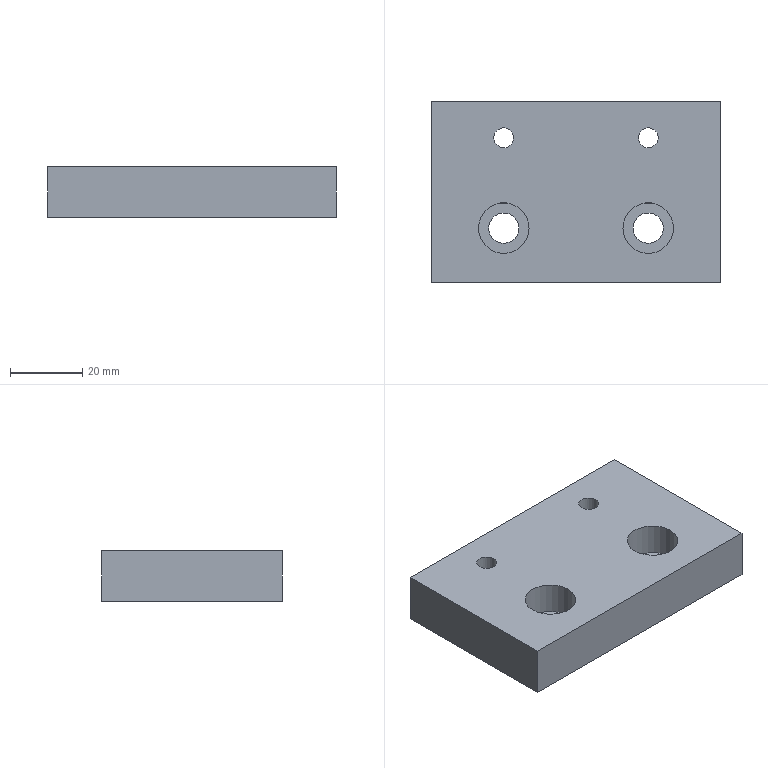Part | STEP file | 1 solid | 18 faces | box 80 x 50 x 14 mm | volume 51452 mm3 | plane 10 | cylinder 8 | commonest cylinder face diameters 5.5 x2 8.4 x2 9 x2 14 x2
STEP:
#1=CARTESIAN_POINT('',(0.,0.,0.));
#2=DIRECTION('',(0.,0.,1.));
#3=DIRECTION('',(1.,0.,0.));
#4=AXIS2_PLACEMENT_3D('',#1,#2,#3);
#5=CARTESIAN_POINT('',(57.147,-30.689,0.));
#6=VERTEX_POINT('',#5);
#7=CARTESIAN_POINT('',(52.947,-30.689,0.));
#8=DIRECTION('',(0.,0.,-1.));
#9=DIRECTION('',(1.,0.,0.));
#10=AXIS2_PLACEMENT_3D('',#7,#8,#9);
#11=CIRCLE('',#10,4.2);
#12=CARTESIAN_POINT('',(0.,0.,0.));
#13=DIRECTION('',(0.,0.,1.));
#14=DIRECTION('',(1.,0.,0.));
#15=AXIS2_PLACEMENT_3D('',#12,#13,#14);
#16=PLANE('',#15);
#17=CARTESIAN_POINT('',(57.147,-30.689));
#18=CARTESIAN_POINT('',(57.147,-37.964));
#19=CARTESIAN_POINT('',(50.847,-34.326));
#20=CARTESIAN_POINT('',(44.547,-30.689));
#21=CARTESIAN_POINT('',(50.847,-27.052));
#22=CARTESIAN_POINT('',(57.147,-23.414));
#23=CARTESIAN_POINT('',(57.147,-30.689));
#24=(BOUNDED_CURVE()B_SPLINE_CURVE(2,(#17,#18,#19,#20,#21,#22,#23),.UNSPECIFIED.,.T.,.F.)B_SPLINE_CURVE_WITH_KNOTS((1,2,2,2,2,1),(-2.094,0.,2.094,4.189,6.283,8.378),.UNSPECIFIED.)CURVE()GEOMETRIC_REPRESENTATION_ITEM()RATIONAL_B_SPLINE_CURVE((1.,0.5,1.,0.5,1.,0.5,1.))REPRESENTATION_ITEM(''));
#25=(GEOMETRIC_REPRESENTATION_CONTEXT(2)PARAMETRIC_REPRESENTATION_CONTEXT()REPRESENTATION_CONTEXT('',''));
#26=DEFINITIONAL_REPRESENTATION('',(#24),#25);
#27=PCURVE('',#16,#26);
#28=CARTESIAN_POINT('',(52.947,-30.689,14.));
#29=DIRECTION('',(0.,0.,1.));
#30=DIRECTION('',(1.,0.,0.));
#31=AXIS2_PLACEMENT_3D('',#28,#29,#30);
#32=CYLINDRICAL_SURFACE('',#31,4.2);
#33=CARTESIAN_POINT('',(6.283,-14.));
#34=DIRECTION('',(-1.,0.));
#35=VECTOR('',#34,1.);
#36=LINE('',#33,#35);
#37=(GEOMETRIC_REPRESENTATION_CONTEXT(2)PARAMETRIC_REPRESENTATION_CONTEXT()REPRESENTATION_CONTEXT('',''));
#38=DEFINITIONAL_REPRESENTATION('',(#36),#37);
#39=PCURVE('',#32,#38);
#40=SURFACE_CURVE('',#11,(#27,#39),.PCURVE_S1.);
#41=EDGE_CURVE('',#6,#6,#40,.T.);
#42=ORIENTED_EDGE('',*,*,#41,.F.);
#43=EDGE_LOOP('',(#42));
#44=FACE_BOUND('',#43,.T.);
#45=CARTESIAN_POINT('',(17.147,-30.689,0.));
#46=VERTEX_POINT('',#45);
#47=CARTESIAN_POINT('',(12.947,-30.689,0.));
#48=DIRECTION('',(0.,0.,-1.));
#49=DIRECTION('',(1.,0.,0.));
#50=AXIS2_PLACEMENT_3D('',#47,#48,#49);
#51=CIRCLE('',#50,4.2);
#52=CARTESIAN_POINT('',(17.147,-30.689));
#53=CARTESIAN_POINT('',(17.147,-37.964));
#54=CARTESIAN_POINT('',(10.847,-34.326));
#55=CARTESIAN_POINT('',(4.547,-30.689));
#56=CARTESIAN_POINT('',(10.847,-27.052));
#57=CARTESIAN_POINT('',(17.147,-23.414));
#58=CARTESIAN_POINT('',(17.147,-30.689));
#59=(BOUNDED_CURVE()B_SPLINE_CURVE(2,(#52,#53,#54,#55,#56,#57,#58),.UNSPECIFIED.,.T.,.F.)B_SPLINE_CURVE_WITH_KNOTS((1,2,2,2,2,1),(-2.094,0.,2.094,4.189,6.283,8.378),.UNSPECIFIED.)CURVE()GEOMETRIC_REPRESENTATION_ITEM()RATIONAL_B_SPLINE_CURVE((1.,0.5,1.,0.5,1.,0.5,1.))REPRESENTATION_ITEM(''));
#60=(GEOMETRIC_REPRESENTATION_CONTEXT(2)PARAMETRIC_REPRESENTATION_CONTEXT()REPRESENTATION_CONTEXT('',''));
#61=DEFINITIONAL_REPRESENTATION('',(#59),#60);
#62=PCURVE('',#16,#61);
#63=CARTESIAN_POINT('',(12.947,-30.689,14.));
#64=DIRECTION('',(0.,0.,1.));
#65=DIRECTION('',(1.,0.,0.));
#66=AXIS2_PLACEMENT_3D('',#63,#64,#65);
#67=CYLINDRICAL_SURFACE('',#66,4.2);
#68=CARTESIAN_POINT('',(6.283,-14.));
#69=DIRECTION('',(-1.,0.));
#70=VECTOR('',#69,1.);
#71=LINE('',#68,#70);
#72=(GEOMETRIC_REPRESENTATION_CONTEXT(2)PARAMETRIC_REPRESENTATION_CONTEXT()REPRESENTATION_CONTEXT('',''));
#73=DEFINITIONAL_REPRESENTATION('',(#71),#72);
#74=PCURVE('',#67,#73);
#75=SURFACE_CURVE('',#51,(#62,#74),.PCURVE_S1.);
#76=EDGE_CURVE('',#46,#46,#75,.T.);
#77=ORIENTED_EDGE('',*,*,#76,.F.);
#78=EDGE_LOOP('',(#77));
#79=FACE_BOUND('',#78,.T.);
#80=CARTESIAN_POINT('',(8.447,-5.689,0.));
#81=VERTEX_POINT('',#80);
#82=CARTESIAN_POINT('',(12.947,-5.689,0.));
#83=DIRECTION('',(0.,0.,-1.));
#84=DIRECTION('',(-1.,0.,0.));
#85=AXIS2_PLACEMENT_3D('',#82,#83,#84);
#86=CIRCLE('',#85,4.5);
#87=CARTESIAN_POINT('',(8.447,-5.689));
#88=CARTESIAN_POINT('',(8.447,2.105));
#89=CARTESIAN_POINT('',(15.197,-1.792));
#90=CARTESIAN_POINT('',(21.947,-5.689));
#91=CARTESIAN_POINT('',(15.197,-9.586));
#92=CARTESIAN_POINT('',(8.447,-13.483));
#93=CARTESIAN_POINT('',(8.447,-5.689));
#94=(BOUNDED_CURVE()B_SPLINE_CURVE(2,(#87,#88,#89,#90,#91,#92,#93),.UNSPECIFIED.,.T.,.F.)B_SPLINE_CURVE_WITH_KNOTS((1,2,2,2,2,1),(-2.094,0.,2.094,4.189,6.283,8.378),.UNSPECIFIED.)CURVE()GEOMETRIC_REPRESENTATION_ITEM()RATIONAL_B_SPLINE_CURVE((1.,0.5,1.,0.5,1.,0.5,1.))REPRESENTATION_ITEM(''));
#95=(GEOMETRIC_REPRESENTATION_CONTEXT(2)PARAMETRIC_REPRESENTATION_CONTEXT()REPRESENTATION_CONTEXT('',''));
#96=DEFINITIONAL_REPRESENTATION('',(#94),#95);
#97=PCURVE('',#16,#96);
#98=CARTESIAN_POINT('',(12.947,-5.689,0.));
#99=DIRECTION('',(0.,0.,-1.));
#100=DIRECTION('',(-1.,0.,0.));
#101=AXIS2_PLACEMENT_3D('',#98,#99,#100);
#102=CYLINDRICAL_SURFACE('',#101,4.5);
#103=CARTESIAN_POINT('',(0.,0.));
#104=DIRECTION('',(1.,0.));
#105=VECTOR('',#104,1.);
#106=LINE('',#103,#105);
#107=(GEOMETRIC_REPRESENTATION_CONTEXT(2)PARAMETRIC_REPRESENTATION_CONTEXT()REPRESENTATION_CONTEXT('',''));
#108=DEFINITIONAL_REPRESENTATION('',(#106),#107);
#109=PCURVE('',#102,#108);
#110=SURFACE_CURVE('',#86,(#97,#109),.PCURVE_S1.);
#111=EDGE_CURVE('',#81,#81,#110,.T.);
#112=ORIENTED_EDGE('',*,*,#111,.F.);
#113=EDGE_LOOP('',(#112));
#114=FACE_BOUND('',#113,.T.);
#115=CARTESIAN_POINT('',(48.447,-5.689,0.));
#116=VERTEX_POINT('',#115);
#117=CARTESIAN_POINT('',(52.947,-5.689,0.));
#118=DIRECTION('',(0.,0.,-1.));
#119=DIRECTION('',(-1.,0.,0.));
#120=AXIS2_PLACEMENT_3D('',#117,#118,#119);
#121=CIRCLE('',#120,4.5);
#122=CARTESIAN_POINT('',(48.447,-5.689));
#123=CARTESIAN_POINT('',(48.447,2.105));
#124=CARTESIAN_POINT('',(55.197,-1.792));
#125=CARTESIAN_POINT('',(61.947,-5.689));
#126=CARTESIAN_POINT('',(55.197,-9.586));
#127=CARTESIAN_POINT('',(48.447,-13.483));
#128=CARTESIAN_POINT('',(48.447,-5.689));
#129=(BOUNDED_CURVE()B_SPLINE_CURVE(2,(#122,#123,#124,#125,#126,#127,#128),.UNSPECIFIED.,.T.,.F.)B_SPLINE_CURVE_WITH_KNOTS((1,2,2,2,2,1),(-2.094,0.,2.094,4.189,6.283,8.378),.UNSPECIFIED.)CURVE()GEOMETRIC_REPRESENTATION_ITEM()RATIONAL_B_SPLINE_CURVE((1.,0.5,1.,0.5,1.,0.5,1.))REPRESENTATION_ITEM(''));
#130=(GEOMETRIC_REPRESENTATION_CONTEXT(2)PARAMETRIC_REPRESENTATION_CONTEXT()REPRESENTATION_CONTEXT('',''));
#131=DEFINITIONAL_REPRESENTATION('',(#129),#130);
#132=PCURVE('',#16,#131);
#133=CARTESIAN_POINT('',(52.947,-5.689,0.));
#134=DIRECTION('',(0.,0.,-1.));
#135=DIRECTION('',(-1.,0.,0.));
#136=AXIS2_PLACEMENT_3D('',#133,#134,#135);
#137=CYLINDRICAL_SURFACE('',#136,4.5);
#138=CARTESIAN_POINT('',(0.,0.));
#139=DIRECTION('',(1.,0.));
#140=VECTOR('',#139,1.);
#141=LINE('',#138,#140);
#142=(GEOMETRIC_REPRESENTATION_CONTEXT(2)PARAMETRIC_REPRESENTATION_CONTEXT()REPRESENTATION_CONTEXT('',''));
#143=DEFINITIONAL_REPRESENTATION('',(#141),#142);
#144=PCURVE('',#137,#143);
#145=SURFACE_CURVE('',#121,(#132,#144),.PCURVE_S1.);
#146=EDGE_CURVE('',#116,#116,#145,.T.);
#147=ORIENTED_EDGE('',*,*,#146,.F.);
#148=EDGE_LOOP('',(#147));
#149=FACE_BOUND('',#148,.T.);
#150=CARTESIAN_POINT('',(72.947,4.311,0.));
#151=VERTEX_POINT('',#150);
#152=CARTESIAN_POINT('',(-7.053,4.311,0.));
#153=VERTEX_POINT('',#152);
#154=CARTESIAN_POINT('',(0.,4.311,0.));
#155=DIRECTION('',(-1.,0.,0.));
#156=VECTOR('',#155,1.);
#157=LINE('',#154,#156);
#158=CARTESIAN_POINT('',(0.,4.311));
#159=DIRECTION('',(-1.,0.));
#160=VECTOR('',#159,1.);
#161=LINE('',#158,#160);
#162=(GEOMETRIC_REPRESENTATION_CONTEXT(2)PARAMETRIC_REPRESENTATION_CONTEXT()REPRESENTATION_CONTEXT('',''));
#163=DEFINITIONAL_REPRESENTATION('',(#161),#162);
#164=PCURVE('',#16,#163);
#165=CARTESIAN_POINT('',(-7.053,4.311,14.));
#166=DIRECTION('',(0.,-1.,0.));
#167=DIRECTION('',(0.,0.,-1.));
#168=AXIS2_PLACEMENT_3D('',#165,#166,#167);
#169=PLANE('',#168);
#170=CARTESIAN_POINT('',(14.,7.053));
#171=DIRECTION('',(0.,-1.));
#172=VECTOR('',#171,1.);
#173=LINE('',#170,#172);
#174=(GEOMETRIC_REPRESENTATION_CONTEXT(2)PARAMETRIC_REPRESENTATION_CONTEXT()REPRESENTATION_CONTEXT('',''));
#175=DEFINITIONAL_REPRESENTATION('',(#173),#174);
#176=PCURVE('',#169,#175);
#177=SURFACE_CURVE('',#157,(#164,#176),.PCURVE_S1.);
#178=EDGE_CURVE('',#151,#153,#177,.T.);
#179=ORIENTED_EDGE('',*,*,#178,.F.);
#180=CARTESIAN_POINT('',(72.947,-45.689,0.));
#181=VERTEX_POINT('',#180);
#182=CARTESIAN_POINT('',(72.947,0.,0.));
#183=DIRECTION('',(0.,1.,0.));
#184=VECTOR('',#183,1.);
#185=LINE('',#182,#184);
#186=CARTESIAN_POINT('',(72.947,0.));
#187=DIRECTION('',(0.,1.));
#188=VECTOR('',#187,1.);
#189=LINE('',#186,#188);
#190=(GEOMETRIC_REPRESENTATION_CONTEXT(2)PARAMETRIC_REPRESENTATION_CONTEXT()REPRESENTATION_CONTEXT('',''));
#191=DEFINITIONAL_REPRESENTATION('',(#189),#190);
#192=PCURVE('',#16,#191);
#193=CARTESIAN_POINT('',(72.947,4.311,14.));
#194=DIRECTION('',(-1.,0.,0.));
#195=DIRECTION('',(0.,0.,1.));
#196=AXIS2_PLACEMENT_3D('',#193,#194,#195);
#197=PLANE('',#196);
#198=CARTESIAN_POINT('',(-14.,-4.311));
#199=DIRECTION('',(0.,1.));
#200=VECTOR('',#199,1.);
#201=LINE('',#198,#200);
#202=(GEOMETRIC_REPRESENTATION_CONTEXT(2)PARAMETRIC_REPRESENTATION_CONTEXT()REPRESENTATION_CONTEXT('',''));
#203=DEFINITIONAL_REPRESENTATION('',(#201),#202);
#204=PCURVE('',#197,#203);
#205=SURFACE_CURVE('',#185,(#192,#204),.PCURVE_S1.);
#206=EDGE_CURVE('',#181,#151,#205,.T.);
#207=ORIENTED_EDGE('',*,*,#206,.F.);
#208=CARTESIAN_POINT('',(-7.053,-45.689,0.));
#209=VERTEX_POINT('',#208);
#210=CARTESIAN_POINT('',(0.,-45.689,0.));
#211=DIRECTION('',(1.,0.,0.));
#212=VECTOR('',#211,1.);
#213=LINE('',#210,#212);
#214=CARTESIAN_POINT('',(0.,-45.689));
#215=DIRECTION('',(1.,0.));
#216=VECTOR('',#215,1.);
#217=LINE('',#214,#216);
#218=(GEOMETRIC_REPRESENTATION_CONTEXT(2)PARAMETRIC_REPRESENTATION_CONTEXT()REPRESENTATION_CONTEXT('',''));
#219=DEFINITIONAL_REPRESENTATION('',(#217),#218);
#220=PCURVE('',#16,#219);
#221=CARTESIAN_POINT('',(-7.053,-45.689,14.));
#222=DIRECTION('',(0.,1.,0.));
#223=DIRECTION('',(0.,0.,1.));
#224=AXIS2_PLACEMENT_3D('',#221,#222,#223);
#225=PLANE('',#224);
#226=CARTESIAN_POINT('',(-14.,7.053));
#227=DIRECTION('',(0.,1.));
#228=VECTOR('',#227,1.);
#229=LINE('',#226,#228);
#230=(GEOMETRIC_REPRESENTATION_CONTEXT(2)PARAMETRIC_REPRESENTATION_CONTEXT()REPRESENTATION_CONTEXT('',''));
#231=DEFINITIONAL_REPRESENTATION('',(#229),#230);
#232=PCURVE('',#225,#231);
#233=SURFACE_CURVE('',#213,(#220,#232),.PCURVE_S1.);
#234=EDGE_CURVE('',#209,#181,#233,.T.);
#235=ORIENTED_EDGE('',*,*,#234,.F.);
#236=CARTESIAN_POINT('',(-7.053,0.,0.));
#237=DIRECTION('',(0.,-1.,0.));
#238=VECTOR('',#237,1.);
#239=LINE('',#236,#238);
#240=CARTESIAN_POINT('',(-7.053,0.));
#241=DIRECTION('',(0.,-1.));
#242=VECTOR('',#241,1.);
#243=LINE('',#240,#242);
#244=(GEOMETRIC_REPRESENTATION_CONTEXT(2)PARAMETRIC_REPRESENTATION_CONTEXT()REPRESENTATION_CONTEXT('',''));
#245=DEFINITIONAL_REPRESENTATION('',(#243),#244);
#246=PCURVE('',#16,#245);
#247=CARTESIAN_POINT('',(-7.053,4.311,14.));
#248=DIRECTION('',(1.,0.,0.));
#249=DIRECTION('',(0.,0.,-1.));
#250=AXIS2_PLACEMENT_3D('',#247,#248,#249);
#251=PLANE('',#250);
#252=CARTESIAN_POINT('',(14.,-4.311));
#253=DIRECTION('',(0.,-1.));
#254=VECTOR('',#253,1.);
#255=LINE('',#252,#254);
#256=(GEOMETRIC_REPRESENTATION_CONTEXT(2)PARAMETRIC_REPRESENTATION_CONTEXT()REPRESENTATION_CONTEXT('',''));
#257=DEFINITIONAL_REPRESENTATION('',(#255),#256);
#258=PCURVE('',#251,#257);
#259=SURFACE_CURVE('',#239,(#246,#258),.PCURVE_S1.);
#260=EDGE_CURVE('',#153,#209,#259,.T.);
#261=ORIENTED_EDGE('',*,*,#260,.F.);
#262=EDGE_LOOP('',(#179,#207,#235,#261));
#263=FACE_BOUND('',#262,.T.);
#264=ADVANCED_FACE('',(#44,#79,#114,#149,#263),#16,.F.);
#265=ORIENTED_EDGE('',*,*,#41,.F.);
#266=CARTESIAN_POINT('',(57.147,-30.689,5.));
#267=VERTEX_POINT('',#266);
#268=CARTESIAN_POINT('',(57.147,-30.689,0.));
#269=CARTESIAN_POINT('',(57.147,-30.689,5.));
#270=B_SPLINE_CURVE_WITH_KNOTS('',1,(#268,#269),.UNSPECIFIED.,.F.,.F.,(2,2),(-14.,-9.),.PIECEWISE_BEZIER_KNOTS.);
#271=CARTESIAN_POINT('',(6.283,0.));
#272=DIRECTION('',(0.,1.));
#273=VECTOR('',#272,1.);
#274=LINE('',#271,#273);
#275=(GEOMETRIC_REPRESENTATION_CONTEXT(2)PARAMETRIC_REPRESENTATION_CONTEXT()REPRESENTATION_CONTEXT('',''));
#276=DEFINITIONAL_REPRESENTATION('',(#274),#275);
#277=PCURVE('',#32,#276);
#278=CARTESIAN_POINT('',(0.,0.));
#279=DIRECTION('',(0.,1.));
#280=VECTOR('',#279,1.);
#281=LINE('',#278,#280);
#282=(GEOMETRIC_REPRESENTATION_CONTEXT(2)PARAMETRIC_REPRESENTATION_CONTEXT()REPRESENTATION_CONTEXT('',''));
#283=DEFINITIONAL_REPRESENTATION('',(#281),#282);
#284=PCURVE('',#32,#283);
#285=SEAM_CURVE('',#270,(#277,#284),.PCURVE_S1.);
#286=EDGE_CURVE('',#6,#267,#285,.T.);
#287=ORIENTED_EDGE('',*,*,#286,.T.);
#288=CARTESIAN_POINT('',(52.947,-30.689,5.));
#289=DIRECTION('',(0.,0.,-1.));
#290=DIRECTION('',(1.,0.,0.));
#291=AXIS2_PLACEMENT_3D('',#288,#289,#290);
#292=CIRCLE('',#291,4.2);
#293=CARTESIAN_POINT('',(6.283,-9.));
#294=DIRECTION('',(-1.,0.));
#295=VECTOR('',#294,1.);
#296=LINE('',#293,#295);
#297=(GEOMETRIC_REPRESENTATION_CONTEXT(2)PARAMETRIC_REPRESENTATION_CONTEXT()REPRESENTATION_CONTEXT('',''));
#298=DEFINITIONAL_REPRESENTATION('',(#296),#297);
#299=PCURVE('',#32,#298);
#300=CARTESIAN_POINT('',(57.147,-30.689,5.));
#301=DIRECTION('',(0.,0.,-1.));
#302=DIRECTION('',(-1.,0.,0.));
#303=AXIS2_PLACEMENT_3D('',#300,#301,#302);
#304=PLANE('',#303);
#305=CARTESIAN_POINT('',(4.2,0.));
#306=DIRECTION('',(-1.,0.));
#307=AXIS2_PLACEMENT_2D('',#305,#306);
#308=CIRCLE('',#307,4.2);
#309=(GEOMETRIC_REPRESENTATION_CONTEXT(2)PARAMETRIC_REPRESENTATION_CONTEXT()REPRESENTATION_CONTEXT('',''));
#310=DEFINITIONAL_REPRESENTATION('',(#308),#309);
#311=PCURVE('',#304,#310);
#312=SURFACE_CURVE('',#292,(#299,#311),.PCURVE_S1.);
#313=EDGE_CURVE('',#267,#267,#312,.T.);
#314=ORIENTED_EDGE('',*,*,#313,.T.);
#315=ORIENTED_EDGE('',*,*,#286,.F.);
#316=EDGE_LOOP('',(#265,#287,#314,#315));
#317=FACE_BOUND('',#316,.F.);
#318=ADVANCED_FACE('',(#317),#32,.F.);
#319=ORIENTED_EDGE('',*,*,#76,.F.);
#320=CARTESIAN_POINT('',(17.147,-30.689,5.));
#321=VERTEX_POINT('',#320);
#322=CARTESIAN_POINT('',(17.147,-30.689,0.));
#323=CARTESIAN_POINT('',(17.147,-30.689,5.));
#324=B_SPLINE_CURVE_WITH_KNOTS('',1,(#322,#323),.UNSPECIFIED.,.F.,.F.,(2,2),(-14.,-9.),.PIECEWISE_BEZIER_KNOTS.);
#325=CARTESIAN_POINT('',(6.283,0.));
#326=DIRECTION('',(0.,1.));
#327=VECTOR('',#326,1.);
#328=LINE('',#325,#327);
#329=(GEOMETRIC_REPRESENTATION_CONTEXT(2)PARAMETRIC_REPRESENTATION_CONTEXT()REPRESENTATION_CONTEXT('',''));
#330=DEFINITIONAL_REPRESENTATION('',(#328),#329);
#331=PCURVE('',#67,#330);
#332=CARTESIAN_POINT('',(0.,0.));
#333=DIRECTION('',(0.,1.));
#334=VECTOR('',#333,1.);
#335=LINE('',#332,#334);
#336=(GEOMETRIC_REPRESENTATION_CONTEXT(2)PARAMETRIC_REPRESENTATION_CONTEXT()REPRESENTATION_CONTEXT('',''));
#337=DEFINITIONAL_REPRESENTATION('',(#335),#336);
#338=PCURVE('',#67,#337);
#339=SEAM_CURVE('',#324,(#331,#338),.PCURVE_S1.);
#340=EDGE_CURVE('',#46,#321,#339,.T.);
#341=ORIENTED_EDGE('',*,*,#340,.T.);
#342=CARTESIAN_POINT('',(12.947,-30.689,5.));
#343=DIRECTION('',(0.,0.,-1.));
#344=DIRECTION('',(1.,0.,0.));
#345=AXIS2_PLACEMENT_3D('',#342,#343,#344);
#346=CIRCLE('',#345,4.2);
#347=CARTESIAN_POINT('',(6.283,-9.));
#348=DIRECTION('',(-1.,0.));
#349=VECTOR('',#348,1.);
#350=LINE('',#347,#349);
#351=(GEOMETRIC_REPRESENTATION_CONTEXT(2)PARAMETRIC_REPRESENTATION_CONTEXT()REPRESENTATION_CONTEXT('',''));
#352=DEFINITIONAL_REPRESENTATION('',(#350),#351);
#353=PCURVE('',#67,#352);
#354=CARTESIAN_POINT('',(17.147,-30.689,5.));
#355=DIRECTION('',(0.,0.,-1.));
#356=DIRECTION('',(-1.,0.,0.));
#357=AXIS2_PLACEMENT_3D('',#354,#355,#356);
#358=PLANE('',#357);
#359=CARTESIAN_POINT('',(4.2,0.));
#360=DIRECTION('',(-1.,0.));
#361=AXIS2_PLACEMENT_2D('',#359,#360);
#362=CIRCLE('',#361,4.2);
#363=(GEOMETRIC_REPRESENTATION_CONTEXT(2)PARAMETRIC_REPRESENTATION_CONTEXT()REPRESENTATION_CONTEXT('',''));
#364=DEFINITIONAL_REPRESENTATION('',(#362),#363);
#365=PCURVE('',#358,#364);
#366=SURFACE_CURVE('',#346,(#353,#365),.PCURVE_S1.);
#367=EDGE_CURVE('',#321,#321,#366,.T.);
#368=ORIENTED_EDGE('',*,*,#367,.T.);
#369=ORIENTED_EDGE('',*,*,#340,.F.);
#370=EDGE_LOOP('',(#319,#341,#368,#369));
#371=FACE_BOUND('',#370,.F.);
#372=ADVANCED_FACE('',(#371),#67,.F.);
#373=CARTESIAN_POINT('',(8.447,-5.689,7.));
#374=VERTEX_POINT('',#373);
#375=CARTESIAN_POINT('',(12.947,-5.689,7.));
#376=DIRECTION('',(0.,0.,-1.));
#377=DIRECTION('',(-1.,0.,0.));
#378=AXIS2_PLACEMENT_3D('',#375,#376,#377);
#379=CIRCLE('',#378,4.5);
#380=CARTESIAN_POINT('',(0.,-7.));
#381=DIRECTION('',(1.,0.));
#382=VECTOR('',#381,1.);
#383=LINE('',#380,#382);
#384=(GEOMETRIC_REPRESENTATION_CONTEXT(2)PARAMETRIC_REPRESENTATION_CONTEXT()REPRESENTATION_CONTEXT('',''));
#385=DEFINITIONAL_REPRESENTATION('',(#383),#384);
#386=PCURVE('',#102,#385);
#387=CARTESIAN_POINT('',(15.697,-5.689,7.));
#388=DIRECTION('',(0.,0.,1.));
#389=DIRECTION('',(1.,0.,0.));
#390=AXIS2_PLACEMENT_3D('',#387,#388,#389);
#391=PLANE('',#390);
#392=CARTESIAN_POINT('',(-7.25,0.));
#393=CARTESIAN_POINT('',(-7.25,7.794));
#394=CARTESIAN_POINT('',(-0.5,3.897));
#395=CARTESIAN_POINT('',(6.25,0.));
#396=CARTESIAN_POINT('',(-0.5,-3.897));
#397=CARTESIAN_POINT('',(-7.25,-7.794));
#398=CARTESIAN_POINT('',(-7.25,0.));
#399=(BOUNDED_CURVE()B_SPLINE_CURVE(2,(#392,#393,#394,#395,#396,#397,#398),.UNSPECIFIED.,.T.,.F.)B_SPLINE_CURVE_WITH_KNOTS((1,2,2,2,2,1),(-2.094,0.,2.094,4.189,6.283,8.378),.UNSPECIFIED.)CURVE()GEOMETRIC_REPRESENTATION_ITEM()RATIONAL_B_SPLINE_CURVE((1.,0.5,1.,0.5,1.,0.5,1.))REPRESENTATION_ITEM(''));
#400=(GEOMETRIC_REPRESENTATION_CONTEXT(2)PARAMETRIC_REPRESENTATION_CONTEXT()REPRESENTATION_CONTEXT('',''));
#401=DEFINITIONAL_REPRESENTATION('',(#399),#400);
#402=PCURVE('',#391,#401);
#403=SURFACE_CURVE('',#379,(#386,#402),.PCURVE_S1.);
#404=EDGE_CURVE('',#374,#374,#403,.T.);
#405=ORIENTED_EDGE('',*,*,#404,.T.);
#406=CARTESIAN_POINT('',(8.447,-5.689,7.));
#407=CARTESIAN_POINT('',(8.447,-5.689,0.));
#408=B_SPLINE_CURVE_WITH_KNOTS('',1,(#406,#407),.UNSPECIFIED.,.F.,.F.,(2,2),(-7.,0.),.PIECEWISE_BEZIER_KNOTS.);
#409=CARTESIAN_POINT('',(6.283,0.));
#410=DIRECTION('',(0.,1.));
#411=VECTOR('',#410,1.);
#412=LINE('',#409,#411);
#413=(GEOMETRIC_REPRESENTATION_CONTEXT(2)PARAMETRIC_REPRESENTATION_CONTEXT()REPRESENTATION_CONTEXT('',''));
#414=DEFINITIONAL_REPRESENTATION('',(#412),#413);
#415=PCURVE('',#102,#414);
#416=CARTESIAN_POINT('',(0.,0.));
#417=DIRECTION('',(0.,1.));
#418=VECTOR('',#417,1.);
#419=LINE('',#416,#418);
#420=(GEOMETRIC_REPRESENTATION_CONTEXT(2)PARAMETRIC_REPRESENTATION_CONTEXT()REPRESENTATION_CONTEXT('',''));
#421=DEFINITIONAL_REPRESENTATION('',(#419),#420);
#422=PCURVE('',#102,#421);
#423=SEAM_CURVE('',#408,(#415,#422),.PCURVE_S1.);
#424=EDGE_CURVE('',#374,#81,#423,.T.);
#425=ORIENTED_EDGE('',*,*,#424,.T.);
#426=ORIENTED_EDGE('',*,*,#111,.F.);
#427=ORIENTED_EDGE('',*,*,#424,.F.);
#428=EDGE_LOOP('',(#405,#425,#426,#427));
#429=FACE_BOUND('',#428,.F.);
#430=ADVANCED_FACE('',(#429),#102,.F.);
#431=CARTESIAN_POINT('',(48.447,-5.689,7.));
#432=VERTEX_POINT('',#431);
#433=CARTESIAN_POINT('',(52.947,-5.689,7.));
#434=DIRECTION('',(0.,0.,-1.));
#435=DIRECTION('',(-1.,0.,0.));
#436=AXIS2_PLACEMENT_3D('',#433,#434,#435);
#437=CIRCLE('',#436,4.5);
#438=CARTESIAN_POINT('',(0.,-7.));
#439=DIRECTION('',(1.,0.));
#440=VECTOR('',#439,1.);
#441=LINE('',#438,#440);
#442=(GEOMETRIC_REPRESENTATION_CONTEXT(2)PARAMETRIC_REPRESENTATION_CONTEXT()REPRESENTATION_CONTEXT('',''));
#443=DEFINITIONAL_REPRESENTATION('',(#441),#442);
#444=PCURVE('',#137,#443);
#445=CARTESIAN_POINT('',(55.697,-5.689,7.));
#446=DIRECTION('',(0.,0.,1.));
#447=DIRECTION('',(1.,0.,0.));
#448=AXIS2_PLACEMENT_3D('',#445,#446,#447);
#449=PLANE('',#448);
#450=CARTESIAN_POINT('',(-7.25,0.));
#451=CARTESIAN_POINT('',(-7.25,7.794));
#452=CARTESIAN_POINT('',(-0.5,3.897));
#453=CARTESIAN_POINT('',(6.25,0.));
#454=CARTESIAN_POINT('',(-0.5,-3.897));
#455=CARTESIAN_POINT('',(-7.25,-7.794));
#456=CARTESIAN_POINT('',(-7.25,0.));
#457=(BOUNDED_CURVE()B_SPLINE_CURVE(2,(#450,#451,#452,#453,#454,#455,#456),.UNSPECIFIED.,.T.,.F.)B_SPLINE_CURVE_WITH_KNOTS((1,2,2,2,2,1),(-2.094,0.,2.094,4.189,6.283,8.378),.UNSPECIFIED.)CURVE()GEOMETRIC_REPRESENTATION_ITEM()RATIONAL_B_SPLINE_CURVE((1.,0.5,1.,0.5,1.,0.5,1.))REPRESENTATION_ITEM(''));
#458=(GEOMETRIC_REPRESENTATION_CONTEXT(2)PARAMETRIC_REPRESENTATION_CONTEXT()REPRESENTATION_CONTEXT('',''));
#459=DEFINITIONAL_REPRESENTATION('',(#457),#458);
#460=PCURVE('',#449,#459);
#461=SURFACE_CURVE('',#437,(#444,#460),.PCURVE_S1.);
#462=EDGE_CURVE('',#432,#432,#461,.T.);
#463=ORIENTED_EDGE('',*,*,#462,.T.);
#464=CARTESIAN_POINT('',(48.447,-5.689,7.));
#465=CARTESIAN_POINT('',(48.447,-5.689,0.));
#466=B_SPLINE_CURVE_WITH_KNOTS('',1,(#464,#465),.UNSPECIFIED.,.F.,.F.,(2,2),(-7.,0.),.PIECEWISE_BEZIER_KNOTS.);
#467=CARTESIAN_POINT('',(6.283,0.));
#468=DIRECTION('',(0.,1.));
#469=VECTOR('',#468,1.);
#470=LINE('',#467,#469);
#471=(GEOMETRIC_REPRESENTATION_CONTEXT(2)PARAMETRIC_REPRESENTATION_CONTEXT()REPRESENTATION_CONTEXT('',''));
#472=DEFINITIONAL_REPRESENTATION('',(#470),#471);
#473=PCURVE('',#137,#472);
#474=CARTESIAN_POINT('',(0.,0.));
#475=DIRECTION('',(0.,1.));
#476=VECTOR('',#475,1.);
#477=LINE('',#474,#476);
#478=(GEOMETRIC_REPRESENTATION_CONTEXT(2)PARAMETRIC_REPRESENTATION_CONTEXT()REPRESENTATION_CONTEXT('',''));
#479=DEFINITIONAL_REPRESENTATION('',(#477),#478);
#480=PCURVE('',#137,#479);
#481=SEAM_CURVE('',#466,(#473,#480),.PCURVE_S1.);
#482=EDGE_CURVE('',#432,#116,#481,.T.);
#483=ORIENTED_EDGE('',*,*,#482,.T.);
#484=ORIENTED_EDGE('',*,*,#146,.F.);
#485=ORIENTED_EDGE('',*,*,#482,.F.);
#486=EDGE_LOOP('',(#463,#483,#484,#485));
#487=FACE_BOUND('',#486,.F.);
#488=ADVANCED_FACE('',(#487),#137,.F.);
#489=CARTESIAN_POINT('',(-7.053,-45.689,14.));
#490=VERTEX_POINT('',#489);
#491=CARTESIAN_POINT('',(-7.053,-45.689,14.));
#492=DIRECTION('',(0.,0.,-1.));
#493=VECTOR('',#492,1.);
#494=LINE('',#491,#493);
#495=CARTESIAN_POINT('',(0.,-50.));
#496=DIRECTION('',(1.,0.));
#497=VECTOR('',#496,1.);
#498=LINE('',#495,#497);
#499=(GEOMETRIC_REPRESENTATION_CONTEXT(2)PARAMETRIC_REPRESENTATION_CONTEXT()REPRESENTATION_CONTEXT('',''));
#500=DEFINITIONAL_REPRESENTATION('',(#498),#499);
#501=PCURVE('',#251,#500);
#502=CARTESIAN_POINT('',(0.,0.));
#503=DIRECTION('',(-1.,0.));
#504=VECTOR('',#503,1.);
#505=LINE('',#502,#504);
#506=(GEOMETRIC_REPRESENTATION_CONTEXT(2)PARAMETRIC_REPRESENTATION_CONTEXT()REPRESENTATION_CONTEXT('',''));
#507=DEFINITIONAL_REPRESENTATION('',(#505),#506);
#508=PCURVE('',#225,#507);
#509=SURFACE_CURVE('',#494,(#501,#508),.PCURVE_S1.);
#510=EDGE_CURVE('',#490,#209,#509,.T.);
#511=ORIENTED_EDGE('',*,*,#510,.F.);
#512=CARTESIAN_POINT('',(-7.053,4.311,14.));
#513=VERTEX_POINT('',#512);
#514=CARTESIAN_POINT('',(-7.053,4.311,14.));
#515=DIRECTION('',(0.,-1.,0.));
#516=VECTOR('',#515,1.);
#517=LINE('',#514,#516);
#518=CARTESIAN_POINT('',(0.,0.));
#519=DIRECTION('',(0.,-1.));
#520=VECTOR('',#519,1.);
#521=LINE('',#518,#520);
#522=(GEOMETRIC_REPRESENTATION_CONTEXT(2)PARAMETRIC_REPRESENTATION_CONTEXT()REPRESENTATION_CONTEXT('',''));
#523=DEFINITIONAL_REPRESENTATION('',(#521),#522);
#524=PCURVE('',#251,#523);
#525=CARTESIAN_POINT('',(0.,0.,14.));
#526=DIRECTION('',(0.,0.,1.));
#527=DIRECTION('',(1.,0.,0.));
#528=AXIS2_PLACEMENT_3D('',#525,#526,#527);
#529=PLANE('',#528);
#530=CARTESIAN_POINT('',(-7.053,4.311));
#531=DIRECTION('',(0.,-1.));
#532=VECTOR('',#531,1.);
#533=LINE('',#530,#532);
#534=(GEOMETRIC_REPRESENTATION_CONTEXT(2)PARAMETRIC_REPRESENTATION_CONTEXT()REPRESENTATION_CONTEXT('',''));
#535=DEFINITIONAL_REPRESENTATION('',(#533),#534);
#536=PCURVE('',#529,#535);
#537=SURFACE_CURVE('',#517,(#524,#536),.PCURVE_S1.);
#538=EDGE_CURVE('',#513,#490,#537,.T.);
#539=ORIENTED_EDGE('',*,*,#538,.F.);
#540=CARTESIAN_POINT('',(-7.053,4.311,14.));
#541=DIRECTION('',(0.,0.,1.));
#542=VECTOR('',#541,1.);
#543=LINE('',#540,#542);
#544=CARTESIAN_POINT('',(0.,0.));
#545=DIRECTION('',(-1.,0.));
#546=VECTOR('',#545,1.);
#547=LINE('',#544,#546);
#548=(GEOMETRIC_REPRESENTATION_CONTEXT(2)PARAMETRIC_REPRESENTATION_CONTEXT()REPRESENTATION_CONTEXT('',''));
#549=DEFINITIONAL_REPRESENTATION('',(#547),#548);
#550=PCURVE('',#251,#549);
#551=CARTESIAN_POINT('',(0.,0.));
#552=DIRECTION('',(-1.,0.));
#553=VECTOR('',#552,1.);
#554=LINE('',#551,#553);
#555=(GEOMETRIC_REPRESENTATION_CONTEXT(2)PARAMETRIC_REPRESENTATION_CONTEXT()REPRESENTATION_CONTEXT('',''));
#556=DEFINITIONAL_REPRESENTATION('',(#554),#555);
#557=PCURVE('',#169,#556);
#558=SURFACE_CURVE('',#543,(#550,#557),.PCURVE_S1.);
#559=EDGE_CURVE('',#153,#513,#558,.T.);
#560=ORIENTED_EDGE('',*,*,#559,.F.);
#561=ORIENTED_EDGE('',*,*,#260,.T.);
#562=EDGE_LOOP('',(#511,#539,#560,#561));
#563=FACE_BOUND('',#562,.T.);
#564=ADVANCED_FACE('',(#563),#251,.F.);
#565=ORIENTED_EDGE('',*,*,#559,.T.);
#566=CARTESIAN_POINT('',(72.947,4.311,14.));
#567=VERTEX_POINT('',#566);
#568=CARTESIAN_POINT('',(-7.053,4.311,14.));
#569=DIRECTION('',(-1.,0.,0.));
#570=VECTOR('',#569,1.);
#571=LINE('',#568,#570);
#572=CARTESIAN_POINT('',(0.,0.));
#573=DIRECTION('',(0.,-1.));
#574=VECTOR('',#573,1.);
#575=LINE('',#572,#574);
#576=(GEOMETRIC_REPRESENTATION_CONTEXT(2)PARAMETRIC_REPRESENTATION_CONTEXT()REPRESENTATION_CONTEXT('',''));
#577=DEFINITIONAL_REPRESENTATION('',(#575),#576);
#578=PCURVE('',#169,#577);
#579=CARTESIAN_POINT('',(-7.053,4.311));
#580=DIRECTION('',(-1.,0.));
#581=VECTOR('',#580,1.);
#582=LINE('',#579,#581);
#583=(GEOMETRIC_REPRESENTATION_CONTEXT(2)PARAMETRIC_REPRESENTATION_CONTEXT()REPRESENTATION_CONTEXT('',''));
#584=DEFINITIONAL_REPRESENTATION('',(#582),#583);
#585=PCURVE('',#529,#584);
#586=SURFACE_CURVE('',#571,(#578,#585),.PCURVE_S1.);
#587=EDGE_CURVE('',#567,#513,#586,.T.);
#588=ORIENTED_EDGE('',*,*,#587,.F.);
#589=CARTESIAN_POINT('',(72.947,4.311,14.));
#590=DIRECTION('',(0.,0.,1.));
#591=VECTOR('',#590,1.);
#592=LINE('',#589,#591);
#593=CARTESIAN_POINT('',(0.,80.));
#594=DIRECTION('',(-1.,0.));
#595=VECTOR('',#594,1.);
#596=LINE('',#593,#595);
#597=(GEOMETRIC_REPRESENTATION_CONTEXT(2)PARAMETRIC_REPRESENTATION_CONTEXT()REPRESENTATION_CONTEXT('',''));
#598=DEFINITIONAL_REPRESENTATION('',(#596),#597);
#599=PCURVE('',#169,#598);
#600=CARTESIAN_POINT('',(0.,0.));
#601=DIRECTION('',(1.,0.));
#602=VECTOR('',#601,1.);
#603=LINE('',#600,#602);
#604=(GEOMETRIC_REPRESENTATION_CONTEXT(2)PARAMETRIC_REPRESENTATION_CONTEXT()REPRESENTATION_CONTEXT('',''));
#605=DEFINITIONAL_REPRESENTATION('',(#603),#604);
#606=PCURVE('',#197,#605);
#607=SURFACE_CURVE('',#592,(#599,#606),.PCURVE_S1.);
#608=EDGE_CURVE('',#151,#567,#607,.T.);
#609=ORIENTED_EDGE('',*,*,#608,.F.);
#610=ORIENTED_EDGE('',*,*,#178,.T.);
#611=EDGE_LOOP('',(#565,#588,#609,#610));
#612=FACE_BOUND('',#611,.T.);
#613=ADVANCED_FACE('',(#612),#169,.F.);
#614=ORIENTED_EDGE('',*,*,#608,.T.);
#615=CARTESIAN_POINT('',(72.947,-45.689,14.));
#616=VERTEX_POINT('',#615);
#617=CARTESIAN_POINT('',(72.947,4.311,14.));
#618=DIRECTION('',(0.,1.,0.));
#619=VECTOR('',#618,1.);
#620=LINE('',#617,#619);
#621=CARTESIAN_POINT('',(0.,0.));
#622=DIRECTION('',(0.,1.));
#623=VECTOR('',#622,1.);
#624=LINE('',#621,#623);
#625=(GEOMETRIC_REPRESENTATION_CONTEXT(2)PARAMETRIC_REPRESENTATION_CONTEXT()REPRESENTATION_CONTEXT('',''));
#626=DEFINITIONAL_REPRESENTATION('',(#624),#625);
#627=PCURVE('',#197,#626);
#628=CARTESIAN_POINT('',(72.947,4.311));
#629=DIRECTION('',(0.,1.));
#630=VECTOR('',#629,1.);
#631=LINE('',#628,#630);
#632=(GEOMETRIC_REPRESENTATION_CONTEXT(2)PARAMETRIC_REPRESENTATION_CONTEXT()REPRESENTATION_CONTEXT('',''));
#633=DEFINITIONAL_REPRESENTATION('',(#631),#632);
#634=PCURVE('',#529,#633);
#635=SURFACE_CURVE('',#620,(#627,#634),.PCURVE_S1.);
#636=EDGE_CURVE('',#616,#567,#635,.T.);
#637=ORIENTED_EDGE('',*,*,#636,.F.);
#638=CARTESIAN_POINT('',(72.947,-45.689,14.));
#639=DIRECTION('',(0.,0.,1.));
#640=VECTOR('',#639,1.);
#641=LINE('',#638,#640);
#642=CARTESIAN_POINT('',(0.,-50.));
#643=DIRECTION('',(1.,0.));
#644=VECTOR('',#643,1.);
#645=LINE('',#642,#644);
#646=(GEOMETRIC_REPRESENTATION_CONTEXT(2)PARAMETRIC_REPRESENTATION_CONTEXT()REPRESENTATION_CONTEXT('',''));
#647=DEFINITIONAL_REPRESENTATION('',(#645),#646);
#648=PCURVE('',#197,#647);
#649=CARTESIAN_POINT('',(0.,80.));
#650=DIRECTION('',(1.,0.));
#651=VECTOR('',#650,1.);
#652=LINE('',#649,#651);
#653=(GEOMETRIC_REPRESENTATION_CONTEXT(2)PARAMETRIC_REPRESENTATION_CONTEXT()REPRESENTATION_CONTEXT('',''));
#654=DEFINITIONAL_REPRESENTATION('',(#652),#653);
#655=PCURVE('',#225,#654);
#656=SURFACE_CURVE('',#641,(#648,#655),.PCURVE_S1.);
#657=EDGE_CURVE('',#181,#616,#656,.T.);
#658=ORIENTED_EDGE('',*,*,#657,.F.);
#659=ORIENTED_EDGE('',*,*,#206,.T.);
#660=EDGE_LOOP('',(#614,#637,#658,#659));
#661=FACE_BOUND('',#660,.T.);
#662=ADVANCED_FACE('',(#661),#197,.F.);
#663=ORIENTED_EDGE('',*,*,#657,.T.);
#664=CARTESIAN_POINT('',(-7.053,-45.689,14.));
#665=DIRECTION('',(1.,0.,0.));
#666=VECTOR('',#665,1.);
#667=LINE('',#664,#666);
#668=CARTESIAN_POINT('',(0.,0.));
#669=DIRECTION('',(0.,1.));
#670=VECTOR('',#669,1.);
#671=LINE('',#668,#670);
#672=(GEOMETRIC_REPRESENTATION_CONTEXT(2)PARAMETRIC_REPRESENTATION_CONTEXT()REPRESENTATION_CONTEXT('',''));
#673=DEFINITIONAL_REPRESENTATION('',(#671),#672);
#674=PCURVE('',#225,#673);
#675=CARTESIAN_POINT('',(-7.053,-45.689));
#676=DIRECTION('',(1.,0.));
#677=VECTOR('',#676,1.);
#678=LINE('',#675,#677);
#679=(GEOMETRIC_REPRESENTATION_CONTEXT(2)PARAMETRIC_REPRESENTATION_CONTEXT()REPRESENTATION_CONTEXT('',''));
#680=DEFINITIONAL_REPRESENTATION('',(#678),#679);
#681=PCURVE('',#529,#680);
#682=SURFACE_CURVE('',#667,(#674,#681),.PCURVE_S1.);
#683=EDGE_CURVE('',#490,#616,#682,.T.);
#684=ORIENTED_EDGE('',*,*,#683,.F.);
#685=ORIENTED_EDGE('',*,*,#510,.T.);
#686=ORIENTED_EDGE('',*,*,#234,.T.);
#687=EDGE_LOOP('',(#663,#684,#685,#686));
#688=FACE_BOUND('',#687,.T.);
#689=ADVANCED_FACE('',(#688),#225,.F.);
#690=ORIENTED_EDGE('',*,*,#313,.T.);
#691=EDGE_LOOP('',(#690));
#692=FACE_BOUND('',#691,.T.);
#693=CARTESIAN_POINT('',(59.947,-30.689,5.));
#694=VERTEX_POINT('',#693);
#695=CARTESIAN_POINT('',(52.947,-30.689,5.));
#696=DIRECTION('',(0.,0.,-1.));
#697=DIRECTION('',(1.,0.,0.));
#698=AXIS2_PLACEMENT_3D('',#695,#696,#697);
#699=CIRCLE('',#698,7.);
#700=CARTESIAN_POINT('',(4.2,0.));
#701=DIRECTION('',(-1.,0.));
#702=AXIS2_PLACEMENT_2D('',#700,#701);
#703=CIRCLE('',#702,7.);
#704=(GEOMETRIC_REPRESENTATION_CONTEXT(2)PARAMETRIC_REPRESENTATION_CONTEXT()REPRESENTATION_CONTEXT('',''));
#705=DEFINITIONAL_REPRESENTATION('',(#703),#704);
#706=PCURVE('',#304,#705);
#707=CARTESIAN_POINT('',(52.947,-30.689,14.));
#708=DIRECTION('',(0.,0.,1.));
#709=DIRECTION('',(1.,0.,0.));
#710=AXIS2_PLACEMENT_3D('',#707,#708,#709);
#711=CYLINDRICAL_SURFACE('',#710,7.);
#712=CARTESIAN_POINT('',(6.283,-9.));
#713=DIRECTION('',(-1.,0.));
#714=VECTOR('',#713,1.);
#715=LINE('',#712,#714);
#716=(GEOMETRIC_REPRESENTATION_CONTEXT(2)PARAMETRIC_REPRESENTATION_CONTEXT()REPRESENTATION_CONTEXT('',''));
#717=DEFINITIONAL_REPRESENTATION('',(#715),#716);
#718=PCURVE('',#711,#717);
#719=SURFACE_CURVE('',#699,(#706,#718),.PCURVE_S1.);
#720=EDGE_CURVE('',#694,#694,#719,.T.);
#721=ORIENTED_EDGE('',*,*,#720,.F.);
#722=EDGE_LOOP('',(#721));
#723=FACE_BOUND('',#722,.T.);
#724=ADVANCED_FACE('',(#692,#723),#304,.F.);
#725=ORIENTED_EDGE('',*,*,#367,.T.);
#726=EDGE_LOOP('',(#725));
#727=FACE_BOUND('',#726,.T.);
#728=CARTESIAN_POINT('',(19.947,-30.689,5.));
#729=VERTEX_POINT('',#728);
#730=CARTESIAN_POINT('',(12.947,-30.689,5.));
#731=DIRECTION('',(0.,0.,-1.));
#732=DIRECTION('',(1.,0.,0.));
#733=AXIS2_PLACEMENT_3D('',#730,#731,#732);
#734=CIRCLE('',#733,7.);
#735=CARTESIAN_POINT('',(4.2,0.));
#736=DIRECTION('',(-1.,0.));
#737=AXIS2_PLACEMENT_2D('',#735,#736);
#738=CIRCLE('',#737,7.);
#739=(GEOMETRIC_REPRESENTATION_CONTEXT(2)PARAMETRIC_REPRESENTATION_CONTEXT()REPRESENTATION_CONTEXT('',''));
#740=DEFINITIONAL_REPRESENTATION('',(#738),#739);
#741=PCURVE('',#358,#740);
#742=CARTESIAN_POINT('',(12.947,-30.689,14.));
#743=DIRECTION('',(0.,0.,1.));
#744=DIRECTION('',(1.,0.,0.));
#745=AXIS2_PLACEMENT_3D('',#742,#743,#744);
#746=CYLINDRICAL_SURFACE('',#745,7.);
#747=CARTESIAN_POINT('',(6.283,-9.));
#748=DIRECTION('',(-1.,0.));
#749=VECTOR('',#748,1.);
#750=LINE('',#747,#749);
#751=(GEOMETRIC_REPRESENTATION_CONTEXT(2)PARAMETRIC_REPRESENTATION_CONTEXT()REPRESENTATION_CONTEXT('',''));
#752=DEFINITIONAL_REPRESENTATION('',(#750),#751);
#753=PCURVE('',#746,#752);
#754=SURFACE_CURVE('',#734,(#741,#753),.PCURVE_S1.);
#755=EDGE_CURVE('',#729,#729,#754,.T.);
#756=ORIENTED_EDGE('',*,*,#755,.F.);
#757=EDGE_LOOP('',(#756));
#758=FACE_BOUND('',#757,.T.);
#759=ADVANCED_FACE('',(#727,#758),#358,.F.);
#760=CARTESIAN_POINT('',(10.197,-5.689,7.));
#761=VERTEX_POINT('',#760);
#762=CARTESIAN_POINT('',(12.947,-5.689,7.));
#763=DIRECTION('',(0.,0.,-1.));
#764=DIRECTION('',(-1.,0.,0.));
#765=AXIS2_PLACEMENT_3D('',#762,#763,#764);
#766=CIRCLE('',#765,2.75);
#767=CARTESIAN_POINT('',(-5.5,0.));
#768=CARTESIAN_POINT('',(-5.5,4.763));
#769=CARTESIAN_POINT('',(-1.375,2.382));
#770=CARTESIAN_POINT('',(2.75,0.));
#771=CARTESIAN_POINT('',(-1.375,-2.382));
#772=CARTESIAN_POINT('',(-5.5,-4.763));
#773=CARTESIAN_POINT('',(-5.5,0.));
#774=(BOUNDED_CURVE()B_SPLINE_CURVE(2,(#767,#768,#769,#770,#771,#772,#773),.UNSPECIFIED.,.T.,.F.)B_SPLINE_CURVE_WITH_KNOTS((1,2,2,2,2,1),(-2.094,0.,2.094,4.189,6.283,8.378),.UNSPECIFIED.)CURVE()GEOMETRIC_REPRESENTATION_ITEM()RATIONAL_B_SPLINE_CURVE((1.,0.5,1.,0.5,1.,0.5,1.))REPRESENTATION_ITEM(''));
#775=(GEOMETRIC_REPRESENTATION_CONTEXT(2)PARAMETRIC_REPRESENTATION_CONTEXT()REPRESENTATION_CONTEXT('',''));
#776=DEFINITIONAL_REPRESENTATION('',(#774),#775);
#777=PCURVE('',#391,#776);
#778=CARTESIAN_POINT('',(12.947,-5.689,0.));
#779=DIRECTION('',(0.,0.,-1.));
#780=DIRECTION('',(-1.,0.,0.));
#781=AXIS2_PLACEMENT_3D('',#778,#779,#780);
#782=CYLINDRICAL_SURFACE('',#781,2.75);
#783=CARTESIAN_POINT('',(0.,-7.));
#784=DIRECTION('',(1.,0.));
#785=VECTOR('',#784,1.);
#786=LINE('',#783,#785);
#787=(GEOMETRIC_REPRESENTATION_CONTEXT(2)PARAMETRIC_REPRESENTATION_CONTEXT()REPRESENTATION_CONTEXT('',''));
#788=DEFINITIONAL_REPRESENTATION('',(#786),#787);
#789=PCURVE('',#782,#788);
#790=SURFACE_CURVE('',#766,(#777,#789),.PCURVE_S1.);
#791=EDGE_CURVE('',#761,#761,#790,.T.);
#792=ORIENTED_EDGE('',*,*,#791,.F.);
#793=EDGE_LOOP('',(#792));
#794=FACE_BOUND('',#793,.T.);
#795=ORIENTED_EDGE('',*,*,#404,.T.);
#796=EDGE_LOOP('',(#795));
#797=FACE_BOUND('',#796,.T.);
#798=ADVANCED_FACE('',(#794,#797),#391,.F.);
#799=CARTESIAN_POINT('',(50.197,-5.689,7.));
#800=VERTEX_POINT('',#799);
#801=CARTESIAN_POINT('',(52.947,-5.689,7.));
#802=DIRECTION('',(0.,0.,-1.));
#803=DIRECTION('',(-1.,0.,0.));
#804=AXIS2_PLACEMENT_3D('',#801,#802,#803);
#805=CIRCLE('',#804,2.75);
#806=CARTESIAN_POINT('',(-5.5,0.));
#807=CARTESIAN_POINT('',(-5.5,4.763));
#808=CARTESIAN_POINT('',(-1.375,2.382));
#809=CARTESIAN_POINT('',(2.75,0.));
#810=CARTESIAN_POINT('',(-1.375,-2.382));
#811=CARTESIAN_POINT('',(-5.5,-4.763));
#812=CARTESIAN_POINT('',(-5.5,0.));
#813=(BOUNDED_CURVE()B_SPLINE_CURVE(2,(#806,#807,#808,#809,#810,#811,#812),.UNSPECIFIED.,.T.,.F.)B_SPLINE_CURVE_WITH_KNOTS((1,2,2,2,2,1),(-2.094,0.,2.094,4.189,6.283,8.378),.UNSPECIFIED.)CURVE()GEOMETRIC_REPRESENTATION_ITEM()RATIONAL_B_SPLINE_CURVE((1.,0.5,1.,0.5,1.,0.5,1.))REPRESENTATION_ITEM(''));
#814=(GEOMETRIC_REPRESENTATION_CONTEXT(2)PARAMETRIC_REPRESENTATION_CONTEXT()REPRESENTATION_CONTEXT('',''));
#815=DEFINITIONAL_REPRESENTATION('',(#813),#814);
#816=PCURVE('',#449,#815);
#817=CARTESIAN_POINT('',(52.947,-5.689,0.));
#818=DIRECTION('',(0.,0.,-1.));
#819=DIRECTION('',(-1.,0.,0.));
#820=AXIS2_PLACEMENT_3D('',#817,#818,#819);
#821=CYLINDRICAL_SURFACE('',#820,2.75);
#822=CARTESIAN_POINT('',(0.,-7.));
#823=DIRECTION('',(1.,0.));
#824=VECTOR('',#823,1.);
#825=LINE('',#822,#824);
#826=(GEOMETRIC_REPRESENTATION_CONTEXT(2)PARAMETRIC_REPRESENTATION_CONTEXT()REPRESENTATION_CONTEXT('',''));
#827=DEFINITIONAL_REPRESENTATION('',(#825),#826);
#828=PCURVE('',#821,#827);
#829=SURFACE_CURVE('',#805,(#816,#828),.PCURVE_S1.);
#830=EDGE_CURVE('',#800,#800,#829,.T.);
#831=ORIENTED_EDGE('',*,*,#830,.F.);
#832=EDGE_LOOP('',(#831));
#833=FACE_BOUND('',#832,.T.);
#834=ORIENTED_EDGE('',*,*,#462,.T.);
#835=EDGE_LOOP('',(#834));
#836=FACE_BOUND('',#835,.T.);
#837=ADVANCED_FACE('',(#833,#836),#449,.F.);
#838=CARTESIAN_POINT('',(50.197,-5.689,14.));
#839=VERTEX_POINT('',#838);
#840=CARTESIAN_POINT('',(52.947,-5.689,14.));
#841=DIRECTION('',(0.,0.,-1.));
#842=DIRECTION('',(-1.,0.,0.));
#843=AXIS2_PLACEMENT_3D('',#840,#841,#842);
#844=CIRCLE('',#843,2.75);
#845=CARTESIAN_POINT('',(50.197,-5.689));
#846=CARTESIAN_POINT('',(50.197,-0.9259));
#847=CARTESIAN_POINT('',(54.322,-3.307));
#848=CARTESIAN_POINT('',(58.447,-5.689));
#849=CARTESIAN_POINT('',(54.322,-8.071));
#850=CARTESIAN_POINT('',(50.197,-10.452));
#851=CARTESIAN_POINT('',(50.197,-5.689));
#852=(BOUNDED_CURVE()B_SPLINE_CURVE(2,(#845,#846,#847,#848,#849,#850,#851),.UNSPECIFIED.,.T.,.F.)B_SPLINE_CURVE_WITH_KNOTS((1,2,2,2,2,1),(-2.094,0.,2.094,4.189,6.283,8.378),.UNSPECIFIED.)CURVE()GEOMETRIC_REPRESENTATION_ITEM()RATIONAL_B_SPLINE_CURVE((1.,0.5,1.,0.5,1.,0.5,1.))REPRESENTATION_ITEM(''));
#853=(GEOMETRIC_REPRESENTATION_CONTEXT(2)PARAMETRIC_REPRESENTATION_CONTEXT()REPRESENTATION_CONTEXT('',''));
#854=DEFINITIONAL_REPRESENTATION('',(#852),#853);
#855=PCURVE('',#529,#854);
#856=CARTESIAN_POINT('',(0.,-14.));
#857=DIRECTION('',(1.,0.));
#858=VECTOR('',#857,1.);
#859=LINE('',#856,#858);
#860=(GEOMETRIC_REPRESENTATION_CONTEXT(2)PARAMETRIC_REPRESENTATION_CONTEXT()REPRESENTATION_CONTEXT('',''));
#861=DEFINITIONAL_REPRESENTATION('',(#859),#860);
#862=PCURVE('',#821,#861);
#863=SURFACE_CURVE('',#844,(#855,#862),.PCURVE_S1.);
#864=EDGE_CURVE('',#839,#839,#863,.T.);
#865=ORIENTED_EDGE('',*,*,#864,.T.);
#866=EDGE_LOOP('',(#865));
#867=FACE_BOUND('',#866,.T.);
#868=CARTESIAN_POINT('',(10.197,-5.689,14.));
#869=VERTEX_POINT('',#868);
#870=CARTESIAN_POINT('',(12.947,-5.689,14.));
#871=DIRECTION('',(0.,0.,-1.));
#872=DIRECTION('',(-1.,0.,0.));
#873=AXIS2_PLACEMENT_3D('',#870,#871,#872);
#874=CIRCLE('',#873,2.75);
#875=CARTESIAN_POINT('',(10.197,-5.689));
#876=CARTESIAN_POINT('',(10.197,-0.9259));
#877=CARTESIAN_POINT('',(14.322,-3.307));
#878=CARTESIAN_POINT('',(18.447,-5.689));
#879=CARTESIAN_POINT('',(14.322,-8.071));
#880=CARTESIAN_POINT('',(10.197,-10.452));
#881=CARTESIAN_POINT('',(10.197,-5.689));
#882=(BOUNDED_CURVE()B_SPLINE_CURVE(2,(#875,#876,#877,#878,#879,#880,#881),.UNSPECIFIED.,.T.,.F.)B_SPLINE_CURVE_WITH_KNOTS((1,2,2,2,2,1),(-2.094,0.,2.094,4.189,6.283,8.378),.UNSPECIFIED.)CURVE()GEOMETRIC_REPRESENTATION_ITEM()RATIONAL_B_SPLINE_CURVE((1.,0.5,1.,0.5,1.,0.5,1.))REPRESENTATION_ITEM(''));
#883=(GEOMETRIC_REPRESENTATION_CONTEXT(2)PARAMETRIC_REPRESENTATION_CONTEXT()REPRESENTATION_CONTEXT('',''));
#884=DEFINITIONAL_REPRESENTATION('',(#882),#883);
#885=PCURVE('',#529,#884);
#886=CARTESIAN_POINT('',(0.,-14.));
#887=DIRECTION('',(1.,0.));
#888=VECTOR('',#887,1.);
#889=LINE('',#886,#888);
#890=(GEOMETRIC_REPRESENTATION_CONTEXT(2)PARAMETRIC_REPRESENTATION_CONTEXT()REPRESENTATION_CONTEXT('',''));
#891=DEFINITIONAL_REPRESENTATION('',(#889),#890);
#892=PCURVE('',#782,#891);
#893=SURFACE_CURVE('',#874,(#885,#892),.PCURVE_S1.);
#894=EDGE_CURVE('',#869,#869,#893,.T.);
#895=ORIENTED_EDGE('',*,*,#894,.T.);
#896=EDGE_LOOP('',(#895));
#897=FACE_BOUND('',#896,.T.);
#898=CARTESIAN_POINT('',(19.947,-30.689,14.));
#899=VERTEX_POINT('',#898);
#900=CARTESIAN_POINT('',(12.947,-30.689,14.));
#901=DIRECTION('',(0.,0.,-1.));
#902=DIRECTION('',(1.,0.,0.));
#903=AXIS2_PLACEMENT_3D('',#900,#901,#902);
#904=CIRCLE('',#903,7.);
#905=CARTESIAN_POINT('',(19.947,-30.689));
#906=CARTESIAN_POINT('',(19.947,-42.813));
#907=CARTESIAN_POINT('',(9.447,-36.751));
#908=CARTESIAN_POINT('',(-1.053,-30.689));
#909=CARTESIAN_POINT('',(9.447,-24.627));
#910=CARTESIAN_POINT('',(19.947,-18.565));
#911=CARTESIAN_POINT('',(19.947,-30.689));
#912=(BOUNDED_CURVE()B_SPLINE_CURVE(2,(#905,#906,#907,#908,#909,#910,#911),.UNSPECIFIED.,.T.,.F.)B_SPLINE_CURVE_WITH_KNOTS((1,2,2,2,2,1),(-2.094,0.,2.094,4.189,6.283,8.378),.UNSPECIFIED.)CURVE()GEOMETRIC_REPRESENTATION_ITEM()RATIONAL_B_SPLINE_CURVE((1.,0.5,1.,0.5,1.,0.5,1.))REPRESENTATION_ITEM(''));
#913=(GEOMETRIC_REPRESENTATION_CONTEXT(2)PARAMETRIC_REPRESENTATION_CONTEXT()REPRESENTATION_CONTEXT('',''));
#914=DEFINITIONAL_REPRESENTATION('',(#912),#913);
#915=PCURVE('',#529,#914);
#916=CARTESIAN_POINT('',(6.283,0.));
#917=DIRECTION('',(-1.,0.));
#918=VECTOR('',#917,1.);
#919=LINE('',#916,#918);
#920=(GEOMETRIC_REPRESENTATION_CONTEXT(2)PARAMETRIC_REPRESENTATION_CONTEXT()REPRESENTATION_CONTEXT('',''));
#921=DEFINITIONAL_REPRESENTATION('',(#919),#920);
#922=PCURVE('',#746,#921);
#923=SURFACE_CURVE('',#904,(#915,#922),.PCURVE_S1.);
#924=EDGE_CURVE('',#899,#899,#923,.T.);
#925=ORIENTED_EDGE('',*,*,#924,.T.);
#926=EDGE_LOOP('',(#925));
#927=FACE_BOUND('',#926,.T.);
#928=CARTESIAN_POINT('',(59.947,-30.689,14.));
#929=VERTEX_POINT('',#928);
#930=CARTESIAN_POINT('',(52.947,-30.689,14.));
#931=DIRECTION('',(0.,0.,-1.));
#932=DIRECTION('',(1.,0.,0.));
#933=AXIS2_PLACEMENT_3D('',#930,#931,#932);
#934=CIRCLE('',#933,7.);
#935=CARTESIAN_POINT('',(59.947,-30.689));
#936=CARTESIAN_POINT('',(59.947,-42.813));
#937=CARTESIAN_POINT('',(49.447,-36.751));
#938=CARTESIAN_POINT('',(38.947,-30.689));
#939=CARTESIAN_POINT('',(49.447,-24.627));
#940=CARTESIAN_POINT('',(59.947,-18.565));
#941=CARTESIAN_POINT('',(59.947,-30.689));
#942=(BOUNDED_CURVE()B_SPLINE_CURVE(2,(#935,#936,#937,#938,#939,#940,#941),.UNSPECIFIED.,.T.,.F.)B_SPLINE_CURVE_WITH_KNOTS((1,2,2,2,2,1),(-2.094,0.,2.094,4.189,6.283,8.378),.UNSPECIFIED.)CURVE()GEOMETRIC_REPRESENTATION_ITEM()RATIONAL_B_SPLINE_CURVE((1.,0.5,1.,0.5,1.,0.5,1.))REPRESENTATION_ITEM(''));
#943=(GEOMETRIC_REPRESENTATION_CONTEXT(2)PARAMETRIC_REPRESENTATION_CONTEXT()REPRESENTATION_CONTEXT('',''));
#944=DEFINITIONAL_REPRESENTATION('',(#942),#943);
#945=PCURVE('',#529,#944);
#946=CARTESIAN_POINT('',(6.283,0.));
#947=DIRECTION('',(-1.,0.));
#948=VECTOR('',#947,1.);
#949=LINE('',#946,#948);
#950=(GEOMETRIC_REPRESENTATION_CONTEXT(2)PARAMETRIC_REPRESENTATION_CONTEXT()REPRESENTATION_CONTEXT('',''));
#951=DEFINITIONAL_REPRESENTATION('',(#949),#950);
#952=PCURVE('',#711,#951);
#953=SURFACE_CURVE('',#934,(#945,#952),.PCURVE_S1.);
#954=EDGE_CURVE('',#929,#929,#953,.T.);
#955=ORIENTED_EDGE('',*,*,#954,.T.);
#956=EDGE_LOOP('',(#955));
#957=FACE_BOUND('',#956,.T.);
#958=ORIENTED_EDGE('',*,*,#636,.T.);
#959=ORIENTED_EDGE('',*,*,#587,.T.);
#960=ORIENTED_EDGE('',*,*,#538,.T.);
#961=ORIENTED_EDGE('',*,*,#683,.T.);
#962=EDGE_LOOP('',(#958,#959,#960,#961));
#963=FACE_BOUND('',#962,.T.);
#964=ADVANCED_FACE('',(#867,#897,#927,#957,#963),#529,.T.);
#965=ORIENTED_EDGE('',*,*,#720,.F.);
#966=CARTESIAN_POINT('',(59.947,-30.689,5.));
#967=CARTESIAN_POINT('',(59.947,-30.689,14.));
#968=B_SPLINE_CURVE_WITH_KNOTS('',1,(#966,#967),.UNSPECIFIED.,.F.,.F.,(2,2),(-9.,0.),.PIECEWISE_BEZIER_KNOTS.);
#969=CARTESIAN_POINT('',(6.283,0.));
#970=DIRECTION('',(0.,1.));
#971=VECTOR('',#970,1.);
#972=LINE('',#969,#971);
#973=(GEOMETRIC_REPRESENTATION_CONTEXT(2)PARAMETRIC_REPRESENTATION_CONTEXT()REPRESENTATION_CONTEXT('',''));
#974=DEFINITIONAL_REPRESENTATION('',(#972),#973);
#975=PCURVE('',#711,#974);
#976=CARTESIAN_POINT('',(0.,0.));
#977=DIRECTION('',(0.,1.));
#978=VECTOR('',#977,1.);
#979=LINE('',#976,#978);
#980=(GEOMETRIC_REPRESENTATION_CONTEXT(2)PARAMETRIC_REPRESENTATION_CONTEXT()REPRESENTATION_CONTEXT('',''));
#981=DEFINITIONAL_REPRESENTATION('',(#979),#980);
#982=PCURVE('',#711,#981);
#983=SEAM_CURVE('',#968,(#975,#982),.PCURVE_S1.);
#984=EDGE_CURVE('',#694,#929,#983,.T.);
#985=ORIENTED_EDGE('',*,*,#984,.T.);
#986=ORIENTED_EDGE('',*,*,#954,.T.);
#987=ORIENTED_EDGE('',*,*,#984,.F.);
#988=EDGE_LOOP('',(#965,#985,#986,#987));
#989=FACE_BOUND('',#988,.F.);
#990=ADVANCED_FACE('',(#989),#711,.F.);
#991=ORIENTED_EDGE('',*,*,#755,.F.);
#992=CARTESIAN_POINT('',(19.947,-30.689,5.));
#993=CARTESIAN_POINT('',(19.947,-30.689,14.));
#994=B_SPLINE_CURVE_WITH_KNOTS('',1,(#992,#993),.UNSPECIFIED.,.F.,.F.,(2,2),(-9.,0.),.PIECEWISE_BEZIER_KNOTS.);
#995=CARTESIAN_POINT('',(6.283,0.));
#996=DIRECTION('',(0.,1.));
#997=VECTOR('',#996,1.);
#998=LINE('',#995,#997);
#999=(GEOMETRIC_REPRESENTATION_CONTEXT(2)PARAMETRIC_REPRESENTATION_CONTEXT()REPRESENTATION_CONTEXT('',''));
#1000=DEFINITIONAL_REPRESENTATION('',(#998),#999);
#1001=PCURVE('',#746,#1000);
#1002=CARTESIAN_POINT('',(0.,0.));
#1003=DIRECTION('',(0.,1.));
#1004=VECTOR('',#1003,1.);
#1005=LINE('',#1002,#1004);
#1006=(GEOMETRIC_REPRESENTATION_CONTEXT(2)PARAMETRIC_REPRESENTATION_CONTEXT()REPRESENTATION_CONTEXT('',''));
#1007=DEFINITIONAL_REPRESENTATION('',(#1005),#1006);
#1008=PCURVE('',#746,#1007);
#1009=SEAM_CURVE('',#994,(#1001,#1008),.PCURVE_S1.);
#1010=EDGE_CURVE('',#729,#899,#1009,.T.);
#1011=ORIENTED_EDGE('',*,*,#1010,.T.);
#1012=ORIENTED_EDGE('',*,*,#924,.T.);
#1013=ORIENTED_EDGE('',*,*,#1010,.F.);
#1014=EDGE_LOOP('',(#991,#1011,#1012,#1013));
#1015=FACE_BOUND('',#1014,.F.);
#1016=ADVANCED_FACE('',(#1015),#746,.F.);
#1017=ORIENTED_EDGE('',*,*,#894,.T.);
#1018=CARTESIAN_POINT('',(10.197,-5.689,14.));
#1019=CARTESIAN_POINT('',(10.197,-5.689,7.));
#1020=B_SPLINE_CURVE_WITH_KNOTS('',1,(#1018,#1019),.UNSPECIFIED.,.F.,.F.,(2,2),(-14.,-7.),.PIECEWISE_BEZIER_KNOTS.);
#1021=CARTESIAN_POINT('',(6.283,0.));
#1022=DIRECTION('',(0.,1.));
#1023=VECTOR('',#1022,1.);
#1024=LINE('',#1021,#1023);
#1025=(GEOMETRIC_REPRESENTATION_CONTEXT(2)PARAMETRIC_REPRESENTATION_CONTEXT()REPRESENTATION_CONTEXT('',''));
#1026=DEFINITIONAL_REPRESENTATION('',(#1024),#1025);
#1027=PCURVE('',#782,#1026);
#1028=CARTESIAN_POINT('',(0.,0.));
#1029=DIRECTION('',(0.,1.));
#1030=VECTOR('',#1029,1.);
#1031=LINE('',#1028,#1030);
#1032=(GEOMETRIC_REPRESENTATION_CONTEXT(2)PARAMETRIC_REPRESENTATION_CONTEXT()REPRESENTATION_CONTEXT('',''));
#1033=DEFINITIONAL_REPRESENTATION('',(#1031),#1032);
#1034=PCURVE('',#782,#1033);
#1035=SEAM_CURVE('',#1020,(#1027,#1034),.PCURVE_S1.);
#1036=EDGE_CURVE('',#869,#761,#1035,.T.);
#1037=ORIENTED_EDGE('',*,*,#1036,.T.);
#1038=ORIENTED_EDGE('',*,*,#791,.F.);
#1039=ORIENTED_EDGE('',*,*,#1036,.F.);
#1040=EDGE_LOOP('',(#1017,#1037,#1038,#1039));
#1041=FACE_BOUND('',#1040,.F.);
#1042=ADVANCED_FACE('',(#1041),#782,.F.);
#1043=ORIENTED_EDGE('',*,*,#864,.T.);
#1044=CARTESIAN_POINT('',(50.197,-5.689,14.));
#1045=CARTESIAN_POINT('',(50.197,-5.689,7.));
#1046=B_SPLINE_CURVE_WITH_KNOTS('',1,(#1044,#1045),.UNSPECIFIED.,.F.,.F.,(2,2),(-14.,-7.),.PIECEWISE_BEZIER_KNOTS.);
#1047=CARTESIAN_POINT('',(6.283,0.));
#1048=DIRECTION('',(0.,1.));
#1049=VECTOR('',#1048,1.);
#1050=LINE('',#1047,#1049);
#1051=(GEOMETRIC_REPRESENTATION_CONTEXT(2)PARAMETRIC_REPRESENTATION_CONTEXT()REPRESENTATION_CONTEXT('',''));
#1052=DEFINITIONAL_REPRESENTATION('',(#1050),#1051);
#1053=PCURVE('',#821,#1052);
#1054=CARTESIAN_POINT('',(0.,0.));
#1055=DIRECTION('',(0.,1.));
#1056=VECTOR('',#1055,1.);
#1057=LINE('',#1054,#1056);
#1058=(GEOMETRIC_REPRESENTATION_CONTEXT(2)PARAMETRIC_REPRESENTATION_CONTEXT()REPRESENTATION_CONTEXT('',''));
#1059=DEFINITIONAL_REPRESENTATION('',(#1057),#1058);
#1060=PCURVE('',#821,#1059);
#1061=SEAM_CURVE('',#1046,(#1053,#1060),.PCURVE_S1.);
#1062=EDGE_CURVE('',#839,#800,#1061,.T.);
#1063=ORIENTED_EDGE('',*,*,#1062,.T.);
#1064=ORIENTED_EDGE('',*,*,#830,.F.);
#1065=ORIENTED_EDGE('',*,*,#1062,.F.);
#1066=EDGE_LOOP('',(#1043,#1063,#1064,#1065));
#1067=FACE_BOUND('',#1066,.F.);
#1068=ADVANCED_FACE('',(#1067),#821,.F.);
#1069=CLOSED_SHELL('',(#264,#318,#372,#430,#488,#564,#613,#662,#689,#724,#759,#798,#837,#964,#990,#1016,#1042,#1068));
#1070=MANIFOLD_SOLID_BREP('',#1069);
#1071=(LENGTH_UNIT()NAMED_UNIT(*)SI_UNIT(.MILLI.,.METRE.));
#1072=UNCERTAINTY_MEASURE_WITH_UNIT(LENGTH_MEASURE(0.000005),#1071,'','');
#1073=(NAMED_UNIT(*)PLANE_ANGLE_UNIT()SI_UNIT($,.RADIAN.));
#1074=(NAMED_UNIT(*)SI_UNIT($,.STERADIAN.)SOLID_ANGLE_UNIT());
#1075=(GEOMETRIC_REPRESENTATION_CONTEXT(3)GLOBAL_UNCERTAINTY_ASSIGNED_CONTEXT((#1072))GLOBAL_UNIT_ASSIGNED_CONTEXT((#1071,#1073,#1074))REPRESENTATION_CONTEXT('',''));
#1076=ADVANCED_BREP_SHAPE_REPRESENTATION('',(#4,#1070),#1075);